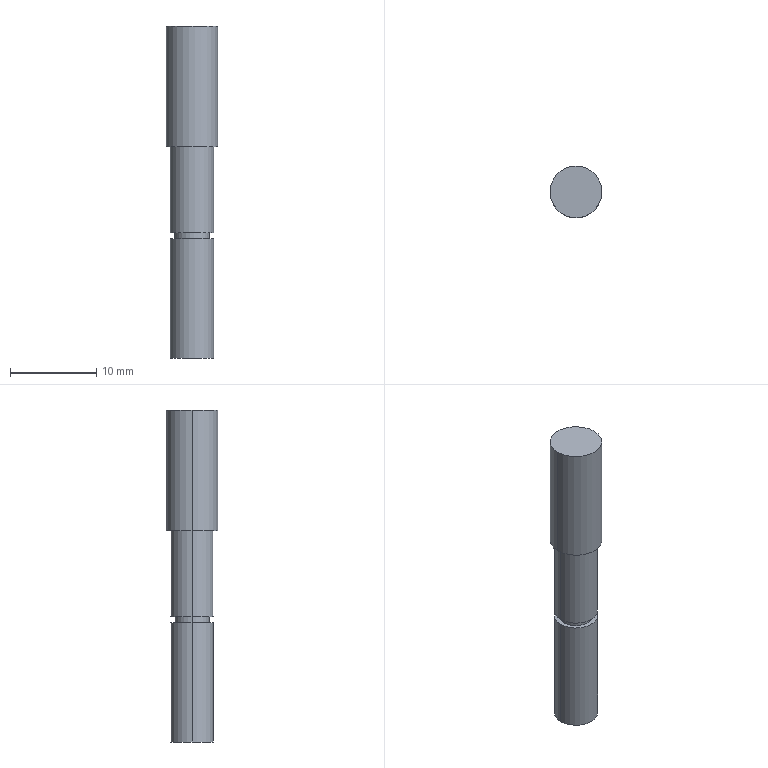Part | SolidWorks | features Extrusion 1, ICE 1, RevCut 1 | 1 solid | 13 faces | box 6 x 6 x 38.5 mm | volume 871.949 mm3 | cylinder 8 | plane 5 | commonest cylinder face diameters 5 x4 4 x2 6 x2
STEP:
#1=CARTESIAN_POINT('',(-2.5,0.,-24.5));
#2=VERTEX_POINT('',#1);
#3=CARTESIAN_POINT('',(2.5,0.,-24.5));
#4=VERTEX_POINT('',#3);
#5=CARTESIAN_POINT('',(0.,0.,-24.5));
#6=DIRECTION('',(0.,0.,-1.));
#7=DIRECTION('',(-1.,0.,0.));
#8=AXIS2_PLACEMENT_3D('',#5,#6,#7);
#9=CIRCLE('',#8,2.5);
#10=EDGE_CURVE('',#2,#4,#9,.T.);
#11=ORIENTED_EDGE('',*,*,#10,.F.);
#12=CARTESIAN_POINT('',(-2.5,0.,-10.7));
#13=VERTEX_POINT('',#12);
#14=CARTESIAN_POINT('',(-2.5,0.,-24.5));
#15=DIRECTION('',(0.,0.,1.));
#16=VECTOR('',#15,1000.);
#17=LINE('',#14,#16);
#18=EDGE_CURVE('',#2,#13,#17,.T.);
#19=ORIENTED_EDGE('',*,*,#18,.T.);
#20=CARTESIAN_POINT('',(2.5,0.,-10.7));
#21=VERTEX_POINT('',#20);
#22=CARTESIAN_POINT('',(0.,0.,-10.7));
#23=DIRECTION('',(0.,0.,1.));
#24=DIRECTION('',(1.,0.,0.));
#25=AXIS2_PLACEMENT_3D('',#22,#23,#24);
#26=CIRCLE('',#25,2.5);
#27=EDGE_CURVE('',#21,#13,#26,.T.);
#28=ORIENTED_EDGE('',*,*,#27,.F.);
#29=CARTESIAN_POINT('',(2.5,0.,-24.5));
#30=DIRECTION('',(0.,0.,1.));
#31=VECTOR('',#30,1000.);
#32=LINE('',#29,#31);
#33=EDGE_CURVE('',#4,#21,#32,.T.);
#34=ORIENTED_EDGE('',*,*,#33,.F.);
#35=EDGE_LOOP('',(#11,#19,#28,#34));
#36=FACE_OUTER_BOUND('',#35,.T.);
#37=CARTESIAN_POINT('',(0.,0.,-24.5));
#38=DIRECTION('',(0.,0.,1.));
#39=DIRECTION('',(1.,0.,0.));
#40=AXIS2_PLACEMENT_3D('',#37,#38,#39);
#41=CYLINDRICAL_SURFACE('',#40,2.5);
#42=ADVANCED_FACE('',(#36),#41,.T.);
#43=CARTESIAN_POINT('',(-2.,0.,-10.));
#44=VERTEX_POINT('',#43);
#45=CARTESIAN_POINT('',(2.,0.,-10.));
#46=VERTEX_POINT('',#45);
#47=CARTESIAN_POINT('',(0.,0.,-10.));
#48=DIRECTION('',(0.,0.,-1.));
#49=DIRECTION('',(-1.,0.,0.));
#50=AXIS2_PLACEMENT_3D('',#47,#48,#49);
#51=CIRCLE('',#50,2.);
#52=EDGE_CURVE('',#44,#46,#51,.T.);
#53=ORIENTED_EDGE('',*,*,#52,.T.);
#54=CARTESIAN_POINT('',(2.,0.,-10.7));
#55=VERTEX_POINT('',#54);
#56=CARTESIAN_POINT('',(2.,0.,-21.475));
#57=DIRECTION('',(0.,0.,-1.));
#58=VECTOR('',#57,1000.);
#59=LINE('',#56,#58);
#60=EDGE_CURVE('',#46,#55,#59,.T.);
#61=ORIENTED_EDGE('',*,*,#60,.T.);
#62=CARTESIAN_POINT('',(-2.,0.,-10.7));
#63=VERTEX_POINT('',#62);
#64=CARTESIAN_POINT('',(0.,0.,-10.7));
#65=DIRECTION('',(0.,0.,-1.));
#66=DIRECTION('',(-1.,0.,0.));
#67=AXIS2_PLACEMENT_3D('',#64,#65,#66);
#68=CIRCLE('',#67,2.);
#69=EDGE_CURVE('',#63,#55,#68,.T.);
#70=ORIENTED_EDGE('',*,*,#69,.F.);
#71=CARTESIAN_POINT('',(-2.,0.,-21.475));
#72=DIRECTION('',(0.,0.,-1.));
#73=VECTOR('',#72,1000.);
#74=LINE('',#71,#73);
#75=EDGE_CURVE('',#44,#63,#74,.T.);
#76=ORIENTED_EDGE('',*,*,#75,.F.);
#77=EDGE_LOOP('',(#53,#61,#70,#76));
#78=FACE_OUTER_BOUND('',#77,.T.);
#79=CARTESIAN_POINT('',(0.,0.,-21.475));
#80=DIRECTION('',(0.,0.,-1.));
#81=DIRECTION('',(-1.,0.,0.));
#82=AXIS2_PLACEMENT_3D('',#79,#80,#81);
#83=CYLINDRICAL_SURFACE('',#82,2.);
#84=ADVANCED_FACE('',(#78),#83,.T.);
#85=CARTESIAN_POINT('',(3.,0.,14.));
#86=VERTEX_POINT('',#85);
#87=CARTESIAN_POINT('',(-3.,0.,14.));
#88=VERTEX_POINT('',#87);
#89=CARTESIAN_POINT('',(0.,0.,14.));
#90=DIRECTION('',(0.,0.,1.));
#91=DIRECTION('',(1.,0.,0.));
#92=AXIS2_PLACEMENT_3D('',#89,#90,#91);
#93=CIRCLE('',#92,3.);
#94=EDGE_CURVE('',#86,#88,#93,.T.);
#95=ORIENTED_EDGE('',*,*,#94,.F.);
#96=CARTESIAN_POINT('',(3.,0.,0.));
#97=VERTEX_POINT('',#96);
#98=CARTESIAN_POINT('',(3.,0.,14.));
#99=DIRECTION('',(0.,0.,-1.));
#100=VECTOR('',#99,1000.);
#101=LINE('',#98,#100);
#102=EDGE_CURVE('',#86,#97,#101,.T.);
#103=ORIENTED_EDGE('',*,*,#102,.T.);
#104=CARTESIAN_POINT('',(-3.,0.,0.));
#105=VERTEX_POINT('',#104);
#106=CARTESIAN_POINT('',(0.,0.,0.));
#107=DIRECTION('',(0.,0.,1.));
#108=DIRECTION('',(1.,0.,0.));
#109=AXIS2_PLACEMENT_3D('',#106,#107,#108);
#110=CIRCLE('',#109,3.);
#111=EDGE_CURVE('',#97,#105,#110,.T.);
#112=ORIENTED_EDGE('',*,*,#111,.T.);
#113=CARTESIAN_POINT('',(-3.,0.,14.));
#114=DIRECTION('',(0.,0.,-1.));
#115=VECTOR('',#114,1000.);
#116=LINE('',#113,#115);
#117=EDGE_CURVE('',#88,#105,#116,.T.);
#118=ORIENTED_EDGE('',*,*,#117,.F.);
#119=EDGE_LOOP('',(#95,#103,#112,#118));
#120=FACE_OUTER_BOUND('',#119,.T.);
#121=CARTESIAN_POINT('',(0.,0.,14.));
#122=DIRECTION('',(0.,0.,-1.));
#123=DIRECTION('',(-1.,0.,0.));
#124=AXIS2_PLACEMENT_3D('',#121,#122,#123);
#125=CYLINDRICAL_SURFACE('',#124,3.);
#126=ADVANCED_FACE('',(#120),#125,.T.);
#127=CARTESIAN_POINT('',(-2.5,0.,-10.));
#128=VERTEX_POINT('',#127);
#129=CARTESIAN_POINT('',(2.5,0.,-10.));
#130=VERTEX_POINT('',#129);
#131=CARTESIAN_POINT('',(0.,0.,-10.));
#132=DIRECTION('',(0.,0.,-1.));
#133=DIRECTION('',(-1.,0.,0.));
#134=AXIS2_PLACEMENT_3D('',#131,#132,#133);
#135=CIRCLE('',#134,2.5);
#136=EDGE_CURVE('',#128,#130,#135,.T.);
#137=ORIENTED_EDGE('',*,*,#136,.F.);
#138=CARTESIAN_POINT('',(-2.5,0.,0.));
#139=VERTEX_POINT('',#138);
#140=CARTESIAN_POINT('',(-2.5,0.,-24.5));
#141=DIRECTION('',(0.,0.,1.));
#142=VECTOR('',#141,1000.);
#143=LINE('',#140,#142);
#144=EDGE_CURVE('',#128,#139,#143,.T.);
#145=ORIENTED_EDGE('',*,*,#144,.T.);
#146=CARTESIAN_POINT('',(2.5,0.,0.));
#147=VERTEX_POINT('',#146);
#148=CARTESIAN_POINT('',(0.,0.,0.));
#149=DIRECTION('',(0.,0.,-1.));
#150=DIRECTION('',(1.,0.,0.));
#151=AXIS2_PLACEMENT_3D('',#148,#149,#150);
#152=CIRCLE('',#151,2.5);
#153=EDGE_CURVE('',#139,#147,#152,.T.);
#154=ORIENTED_EDGE('',*,*,#153,.T.);
#155=CARTESIAN_POINT('',(2.5,0.,-24.5));
#156=DIRECTION('',(0.,0.,1.));
#157=VECTOR('',#156,1000.);
#158=LINE('',#155,#157);
#159=EDGE_CURVE('',#130,#147,#158,.T.);
#160=ORIENTED_EDGE('',*,*,#159,.F.);
#161=EDGE_LOOP('',(#137,#145,#154,#160));
#162=FACE_OUTER_BOUND('',#161,.T.);
#163=CARTESIAN_POINT('',(0.,0.,-24.5));
#164=DIRECTION('',(0.,0.,1.));
#165=DIRECTION('',(1.,0.,0.));
#166=AXIS2_PLACEMENT_3D('',#163,#164,#165);
#167=CYLINDRICAL_SURFACE('',#166,2.5);
#168=ADVANCED_FACE('',(#162),#167,.T.);
#169=ORIENTED_EDGE('',*,*,#144,.F.);
#170=CARTESIAN_POINT('',(0.,0.,-10.));
#171=DIRECTION('',(0.,0.,-1.));
#172=DIRECTION('',(-1.,0.,0.));
#173=AXIS2_PLACEMENT_3D('',#170,#171,#172);
#174=CIRCLE('',#173,2.5);
#175=EDGE_CURVE('',#130,#128,#174,.T.);
#176=ORIENTED_EDGE('',*,*,#175,.F.);
#177=ORIENTED_EDGE('',*,*,#159,.T.);
#178=CARTESIAN_POINT('',(0.,0.,0.));
#179=DIRECTION('',(0.,0.,-1.));
#180=DIRECTION('',(1.,0.,0.));
#181=AXIS2_PLACEMENT_3D('',#178,#179,#180);
#182=CIRCLE('',#181,2.5);
#183=EDGE_CURVE('',#147,#139,#182,.T.);
#184=ORIENTED_EDGE('',*,*,#183,.T.);
#185=EDGE_LOOP('',(#169,#176,#177,#184));
#186=FACE_OUTER_BOUND('',#185,.T.);
#187=CARTESIAN_POINT('',(0.,0.,-24.5));
#188=DIRECTION('',(0.,0.,1.));
#189=DIRECTION('',(1.,0.,0.));
#190=AXIS2_PLACEMENT_3D('',#187,#188,#189);
#191=CYLINDRICAL_SURFACE('',#190,2.5);
#192=ADVANCED_FACE('',(#186),#191,.T.);
#193=CARTESIAN_POINT('',(0.,0.,0.));
#194=DIRECTION('',(0.,0.,1.));
#195=DIRECTION('',(1.,0.,0.));
#196=AXIS2_PLACEMENT_3D('',#193,#194,#195);
#197=CIRCLE('',#196,3.);
#198=EDGE_CURVE('',#105,#97,#197,.T.);
#199=ORIENTED_EDGE('',*,*,#198,.F.);
#200=ORIENTED_EDGE('',*,*,#111,.F.);
#201=EDGE_LOOP('',(#199,#200));
#202=FACE_OUTER_BOUND('',#201,.T.);
#203=ORIENTED_EDGE('',*,*,#183,.F.);
#204=ORIENTED_EDGE('',*,*,#153,.F.);
#205=EDGE_LOOP('',(#203,#204));
#206=FACE_BOUND('',#205,.T.);
#207=CARTESIAN_POINT('',(0.,0.,0.));
#208=DIRECTION('',(0.,0.,1.));
#209=DIRECTION('',(1.,0.,0.));
#210=AXIS2_PLACEMENT_3D('',#207,#208,#209);
#211=PLANE('',#210);
#212=ADVANCED_FACE('',(#202,#206),#211,.F.);
#213=ORIENTED_EDGE('',*,*,#102,.F.);
#214=CARTESIAN_POINT('',(0.,0.,14.));
#215=DIRECTION('',(0.,0.,1.));
#216=DIRECTION('',(1.,0.,0.));
#217=AXIS2_PLACEMENT_3D('',#214,#215,#216);
#218=CIRCLE('',#217,3.);
#219=EDGE_CURVE('',#88,#86,#218,.T.);
#220=ORIENTED_EDGE('',*,*,#219,.F.);
#221=ORIENTED_EDGE('',*,*,#117,.T.);
#222=ORIENTED_EDGE('',*,*,#198,.T.);
#223=EDGE_LOOP('',(#213,#220,#221,#222));
#224=FACE_OUTER_BOUND('',#223,.T.);
#225=CARTESIAN_POINT('',(0.,0.,14.));
#226=DIRECTION('',(0.,0.,-1.));
#227=DIRECTION('',(-1.,0.,0.));
#228=AXIS2_PLACEMENT_3D('',#225,#226,#227);
#229=CYLINDRICAL_SURFACE('',#228,3.);
#230=ADVANCED_FACE('',(#224),#229,.T.);
#231=ORIENTED_EDGE('',*,*,#219,.T.);
#232=ORIENTED_EDGE('',*,*,#94,.T.);
#233=EDGE_LOOP('',(#231,#232));
#234=FACE_OUTER_BOUND('',#233,.T.);
#235=CARTESIAN_POINT('',(0.,0.,14.));
#236=DIRECTION('',(0.,0.,1.));
#237=DIRECTION('',(1.,0.,0.));
#238=AXIS2_PLACEMENT_3D('',#235,#236,#237);
#239=PLANE('',#238);
#240=ADVANCED_FACE('',(#234),#239,.T.);
#241=ORIENTED_EDGE('',*,*,#69,.T.);
#242=CARTESIAN_POINT('',(0.,0.,-10.7));
#243=DIRECTION('',(0.,0.,-1.));
#244=DIRECTION('',(-1.,0.,0.));
#245=AXIS2_PLACEMENT_3D('',#242,#243,#244);
#246=CIRCLE('',#245,2.);
#247=EDGE_CURVE('',#55,#63,#246,.T.);
#248=ORIENTED_EDGE('',*,*,#247,.T.);
#249=EDGE_LOOP('',(#241,#248));
#250=FACE_BOUND('',#249,.T.);
#251=ORIENTED_EDGE('',*,*,#27,.T.);
#252=CARTESIAN_POINT('',(0.,0.,-10.7));
#253=DIRECTION('',(0.,0.,1.));
#254=DIRECTION('',(1.,0.,0.));
#255=AXIS2_PLACEMENT_3D('',#252,#253,#254);
#256=CIRCLE('',#255,2.5);
#257=EDGE_CURVE('',#13,#21,#256,.T.);
#258=ORIENTED_EDGE('',*,*,#257,.T.);
#259=EDGE_LOOP('',(#251,#258));
#260=FACE_OUTER_BOUND('',#259,.T.);
#261=CARTESIAN_POINT('',(2.,0.,-10.7));
#262=DIRECTION('',(0.,0.,1.));
#263=DIRECTION('',(1.,0.,0.));
#264=AXIS2_PLACEMENT_3D('',#261,#262,#263);
#265=PLANE('',#264);
#266=ADVANCED_FACE('',(#250,#260),#265,.T.);
#267=ORIENTED_EDGE('',*,*,#52,.F.);
#268=CARTESIAN_POINT('',(0.,0.,-10.));
#269=DIRECTION('',(0.,0.,-1.));
#270=DIRECTION('',(-1.,0.,0.));
#271=AXIS2_PLACEMENT_3D('',#268,#269,#270);
#272=CIRCLE('',#271,2.);
#273=EDGE_CURVE('',#46,#44,#272,.T.);
#274=ORIENTED_EDGE('',*,*,#273,.F.);
#275=EDGE_LOOP('',(#267,#274));
#276=FACE_BOUND('',#275,.T.);
#277=ORIENTED_EDGE('',*,*,#175,.T.);
#278=ORIENTED_EDGE('',*,*,#136,.T.);
#279=EDGE_LOOP('',(#277,#278));
#280=FACE_OUTER_BOUND('',#279,.T.);
#281=CARTESIAN_POINT('',(2.,0.,-10.));
#282=DIRECTION('',(0.,0.,-1.));
#283=DIRECTION('',(-1.,0.,0.));
#284=AXIS2_PLACEMENT_3D('',#281,#282,#283);
#285=PLANE('',#284);
#286=ADVANCED_FACE('',(#276,#280),#285,.T.);
#287=ORIENTED_EDGE('',*,*,#60,.F.);
#288=ORIENTED_EDGE('',*,*,#273,.T.);
#289=ORIENTED_EDGE('',*,*,#75,.T.);
#290=ORIENTED_EDGE('',*,*,#247,.F.);
#291=EDGE_LOOP('',(#287,#288,#289,#290));
#292=FACE_OUTER_BOUND('',#291,.T.);
#293=CARTESIAN_POINT('',(0.,0.,-21.475));
#294=DIRECTION('',(0.,0.,-1.));
#295=DIRECTION('',(-1.,0.,0.));
#296=AXIS2_PLACEMENT_3D('',#293,#294,#295);
#297=CYLINDRICAL_SURFACE('',#296,2.);
#298=ADVANCED_FACE('',(#292),#297,.T.);
#299=CARTESIAN_POINT('',(0.,0.,-24.5));
#300=DIRECTION('',(0.,0.,-1.));
#301=DIRECTION('',(-1.,0.,0.));
#302=AXIS2_PLACEMENT_3D('',#299,#300,#301);
#303=CIRCLE('',#302,2.5);
#304=EDGE_CURVE('',#4,#2,#303,.T.);
#305=ORIENTED_EDGE('',*,*,#304,.T.);
#306=ORIENTED_EDGE('',*,*,#10,.T.);
#307=EDGE_LOOP('',(#305,#306));
#308=FACE_OUTER_BOUND('',#307,.T.);
#309=CARTESIAN_POINT('',(0.,0.,-24.5));
#310=DIRECTION('',(0.,0.,-1.));
#311=DIRECTION('',(-1.,0.,0.));
#312=AXIS2_PLACEMENT_3D('',#309,#310,#311);
#313=PLANE('',#312);
#314=ADVANCED_FACE('',(#308),#313,.T.);
#315=ORIENTED_EDGE('',*,*,#18,.F.);
#316=ORIENTED_EDGE('',*,*,#304,.F.);
#317=ORIENTED_EDGE('',*,*,#33,.T.);
#318=ORIENTED_EDGE('',*,*,#257,.F.);
#319=EDGE_LOOP('',(#315,#316,#317,#318));
#320=FACE_OUTER_BOUND('',#319,.T.);
#321=CARTESIAN_POINT('',(0.,0.,-24.5));
#322=DIRECTION('',(0.,0.,1.));
#323=DIRECTION('',(1.,0.,0.));
#324=AXIS2_PLACEMENT_3D('',#321,#322,#323);
#325=CYLINDRICAL_SURFACE('',#324,2.5);
#326=ADVANCED_FACE('',(#320),#325,.T.);
#327=CLOSED_SHELL('',(#42,#84,#126,#168,#192,#212,#230,#240,#266,#286,#298,#314,#326));
#328=MANIFOLD_SOLID_BREP('',#327);
#329=CARTESIAN_POINT('',(0.,0.,0.));
#330=DIRECTION('',(0.,0.,1.));
#331=DIRECTION('',(1.,0.,0.));
#332=AXIS2_PLACEMENT_3D('',#329,#330,#331);
#333=(LENGTH_UNIT()NAMED_UNIT(*)SI_UNIT(.MILLI.,.METRE.));
#334=UNCERTAINTY_MEASURE_WITH_UNIT(LENGTH_MEASURE(0.00001),#333,'','');
#335=(NAMED_UNIT(*)PLANE_ANGLE_UNIT()SI_UNIT($,.RADIAN.));
#336=(NAMED_UNIT(*)SI_UNIT($,.STERADIAN.)SOLID_ANGLE_UNIT());
#337=(GEOMETRIC_REPRESENTATION_CONTEXT(3)GLOBAL_UNCERTAINTY_ASSIGNED_CONTEXT((#334))GLOBAL_UNIT_ASSIGNED_CONTEXT((#333,#335,#336))REPRESENTATION_CONTEXT('',''));
#338=ADVANCED_BREP_SHAPE_REPRESENTATION('',(#328,#332),#337);